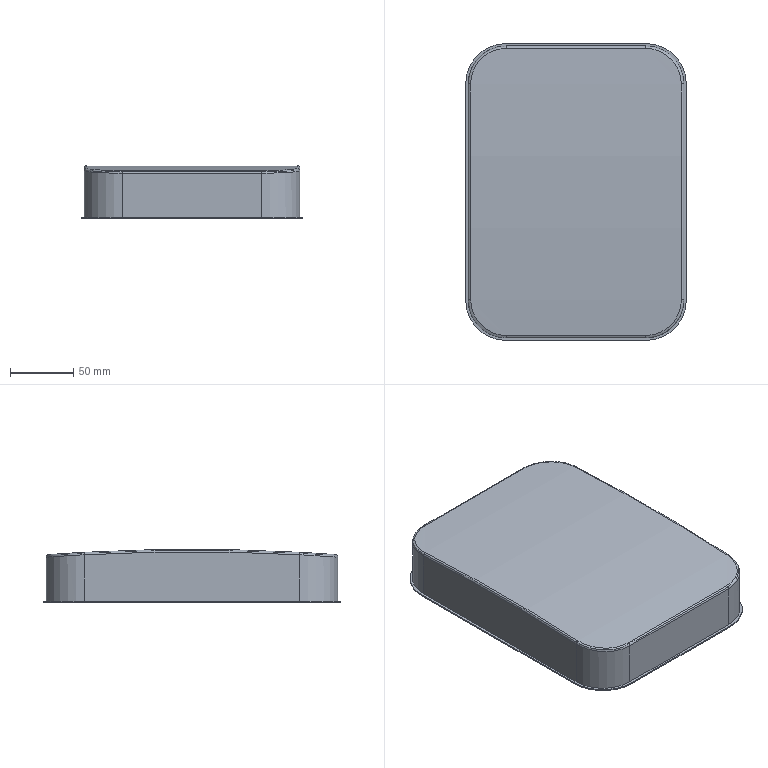Part | SolidWorks | features ICE 2, Extrusion 1, Fillet 1, Shell 1 | 1 solid | 36 faces | box 174 x 234 x 41.94 mm | volume 67886 mm3 | cylinder 16 | plane 14 | spline 4 | torus 2 | commonest cylinder face diameters 58 x4 60 x4 64 x4 4 x2 2998 x1 3000 x1